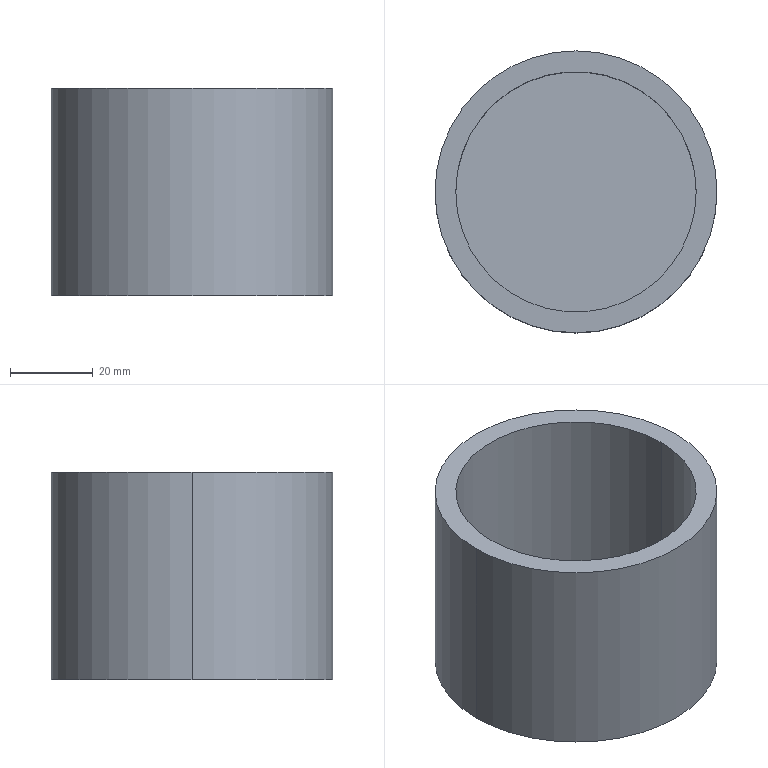Part | SolidWorks | features Extrusion 1, Shell 1 | 1 solid | 7 faces | box 68 x 68 x 50 mm | volume 62690 mm3 | cylinder 4 | plane 3 | commonest cylinder face diameters 58 x2 68 x2
STEP:
#1=CARTESIAN_POINT('',(-29.,0.,50.));
#2=VERTEX_POINT('',#1);
#3=CARTESIAN_POINT('',(29.,0.,50.));
#4=VERTEX_POINT('',#3);
#5=CARTESIAN_POINT('',(0.,0.,50.));
#6=DIRECTION('',(0.,0.,1.));
#7=DIRECTION('',(1.,0.,0.));
#8=AXIS2_PLACEMENT_3D('',#5,#6,#7);
#9=CIRCLE('',#8,29.);
#10=EDGE_CURVE('',#2,#4,#9,.T.);
#11=ORIENTED_EDGE('',*,*,#10,.T.);
#12=CARTESIAN_POINT('',(29.,0.,5.));
#13=VERTEX_POINT('',#12);
#14=CARTESIAN_POINT('',(29.,0.,50.));
#15=DIRECTION('',(0.,0.,-1.));
#16=VECTOR('',#15,1000.);
#17=LINE('',#14,#16);
#18=EDGE_CURVE('',#4,#13,#17,.T.);
#19=ORIENTED_EDGE('',*,*,#18,.T.);
#20=CARTESIAN_POINT('',(-29.,0.,5.));
#21=VERTEX_POINT('',#20);
#22=CARTESIAN_POINT('',(0.,0.,5.));
#23=DIRECTION('',(0.,0.,1.));
#24=DIRECTION('',(1.,0.,0.));
#25=AXIS2_PLACEMENT_3D('',#22,#23,#24);
#26=CIRCLE('',#25,29.);
#27=EDGE_CURVE('',#21,#13,#26,.T.);
#28=ORIENTED_EDGE('',*,*,#27,.F.);
#29=CARTESIAN_POINT('',(-29.,0.,50.));
#30=DIRECTION('',(0.,0.,-1.));
#31=VECTOR('',#30,1000.);
#32=LINE('',#29,#31);
#33=EDGE_CURVE('',#2,#21,#32,.T.);
#34=ORIENTED_EDGE('',*,*,#33,.F.);
#35=EDGE_LOOP('',(#11,#19,#28,#34));
#36=FACE_OUTER_BOUND('',#35,.T.);
#37=CARTESIAN_POINT('',(0.,0.,50.));
#38=DIRECTION('',(0.,0.,-1.));
#39=DIRECTION('',(-1.,0.,0.));
#40=AXIS2_PLACEMENT_3D('',#37,#38,#39);
#41=CYLINDRICAL_SURFACE('',#40,29.);
#42=ADVANCED_FACE('',(#36),#41,.F.);
#43=CARTESIAN_POINT('',(34.,0.,50.));
#44=VERTEX_POINT('',#43);
#45=CARTESIAN_POINT('',(-34.,0.,50.));
#46=VERTEX_POINT('',#45);
#47=CARTESIAN_POINT('',(0.,0.,50.));
#48=DIRECTION('',(0.,0.,1.));
#49=DIRECTION('',(1.,0.,0.));
#50=AXIS2_PLACEMENT_3D('',#47,#48,#49);
#51=CIRCLE('',#50,34.);
#52=EDGE_CURVE('',#44,#46,#51,.T.);
#53=ORIENTED_EDGE('',*,*,#52,.F.);
#54=CARTESIAN_POINT('',(34.,0.,0.));
#55=VERTEX_POINT('',#54);
#56=CARTESIAN_POINT('',(34.,0.,50.));
#57=DIRECTION('',(0.,0.,-1.));
#58=VECTOR('',#57,1000.);
#59=LINE('',#56,#58);
#60=EDGE_CURVE('',#44,#55,#59,.T.);
#61=ORIENTED_EDGE('',*,*,#60,.T.);
#62=CARTESIAN_POINT('',(-34.,0.,0.));
#63=VERTEX_POINT('',#62);
#64=CARTESIAN_POINT('',(0.,0.,0.));
#65=DIRECTION('',(0.,0.,1.));
#66=DIRECTION('',(1.,0.,0.));
#67=AXIS2_PLACEMENT_3D('',#64,#65,#66);
#68=CIRCLE('',#67,34.);
#69=EDGE_CURVE('',#55,#63,#68,.T.);
#70=ORIENTED_EDGE('',*,*,#69,.T.);
#71=CARTESIAN_POINT('',(-34.,0.,50.));
#72=DIRECTION('',(0.,0.,-1.));
#73=VECTOR('',#72,1000.);
#74=LINE('',#71,#73);
#75=EDGE_CURVE('',#46,#63,#74,.T.);
#76=ORIENTED_EDGE('',*,*,#75,.F.);
#77=EDGE_LOOP('',(#53,#61,#70,#76));
#78=FACE_OUTER_BOUND('',#77,.T.);
#79=CARTESIAN_POINT('',(0.,0.,50.));
#80=DIRECTION('',(0.,0.,-1.));
#81=DIRECTION('',(-1.,0.,0.));
#82=AXIS2_PLACEMENT_3D('',#79,#80,#81);
#83=CYLINDRICAL_SURFACE('',#82,34.);
#84=ADVANCED_FACE('',(#78),#83,.T.);
#85=ORIENTED_EDGE('',*,*,#60,.F.);
#86=CARTESIAN_POINT('',(0.,0.,50.));
#87=DIRECTION('',(0.,0.,1.));
#88=DIRECTION('',(1.,0.,0.));
#89=AXIS2_PLACEMENT_3D('',#86,#87,#88);
#90=CIRCLE('',#89,34.);
#91=EDGE_CURVE('',#46,#44,#90,.T.);
#92=ORIENTED_EDGE('',*,*,#91,.F.);
#93=ORIENTED_EDGE('',*,*,#75,.T.);
#94=CARTESIAN_POINT('',(0.,0.,0.));
#95=DIRECTION('',(0.,0.,1.));
#96=DIRECTION('',(1.,0.,0.));
#97=AXIS2_PLACEMENT_3D('',#94,#95,#96);
#98=CIRCLE('',#97,34.);
#99=EDGE_CURVE('',#63,#55,#98,.T.);
#100=ORIENTED_EDGE('',*,*,#99,.T.);
#101=EDGE_LOOP('',(#85,#92,#93,#100));
#102=FACE_OUTER_BOUND('',#101,.T.);
#103=CARTESIAN_POINT('',(0.,0.,50.));
#104=DIRECTION('',(0.,0.,-1.));
#105=DIRECTION('',(-1.,0.,0.));
#106=AXIS2_PLACEMENT_3D('',#103,#104,#105);
#107=CYLINDRICAL_SURFACE('',#106,34.);
#108=ADVANCED_FACE('',(#102),#107,.T.);
#109=ORIENTED_EDGE('',*,*,#10,.F.);
#110=CARTESIAN_POINT('',(0.,0.,50.));
#111=DIRECTION('',(0.,0.,1.));
#112=DIRECTION('',(1.,0.,0.));
#113=AXIS2_PLACEMENT_3D('',#110,#111,#112);
#114=CIRCLE('',#113,29.);
#115=EDGE_CURVE('',#4,#2,#114,.T.);
#116=ORIENTED_EDGE('',*,*,#115,.F.);
#117=EDGE_LOOP('',(#109,#116));
#118=FACE_BOUND('',#117,.T.);
#119=ORIENTED_EDGE('',*,*,#91,.T.);
#120=ORIENTED_EDGE('',*,*,#52,.T.);
#121=EDGE_LOOP('',(#119,#120));
#122=FACE_OUTER_BOUND('',#121,.T.);
#123=CARTESIAN_POINT('',(0.,0.,50.));
#124=DIRECTION('',(0.,0.,1.));
#125=DIRECTION('',(1.,0.,0.));
#126=AXIS2_PLACEMENT_3D('',#123,#124,#125);
#127=PLANE('',#126);
#128=ADVANCED_FACE('',(#118,#122),#127,.T.);
#129=ORIENTED_EDGE('',*,*,#99,.F.);
#130=ORIENTED_EDGE('',*,*,#69,.F.);
#131=EDGE_LOOP('',(#129,#130));
#132=FACE_OUTER_BOUND('',#131,.T.);
#133=CARTESIAN_POINT('',(0.,0.,0.));
#134=DIRECTION('',(0.,0.,1.));
#135=DIRECTION('',(1.,0.,0.));
#136=AXIS2_PLACEMENT_3D('',#133,#134,#135);
#137=PLANE('',#136);
#138=ADVANCED_FACE('',(#132),#137,.F.);
#139=ORIENTED_EDGE('',*,*,#18,.F.);
#140=ORIENTED_EDGE('',*,*,#115,.T.);
#141=ORIENTED_EDGE('',*,*,#33,.T.);
#142=CARTESIAN_POINT('',(0.,0.,5.));
#143=DIRECTION('',(0.,0.,1.));
#144=DIRECTION('',(1.,0.,0.));
#145=AXIS2_PLACEMENT_3D('',#142,#143,#144);
#146=CIRCLE('',#145,29.);
#147=EDGE_CURVE('',#13,#21,#146,.T.);
#148=ORIENTED_EDGE('',*,*,#147,.F.);
#149=EDGE_LOOP('',(#139,#140,#141,#148));
#150=FACE_OUTER_BOUND('',#149,.T.);
#151=CARTESIAN_POINT('',(0.,0.,50.));
#152=DIRECTION('',(0.,0.,-1.));
#153=DIRECTION('',(-1.,0.,0.));
#154=AXIS2_PLACEMENT_3D('',#151,#152,#153);
#155=CYLINDRICAL_SURFACE('',#154,29.);
#156=ADVANCED_FACE('',(#150),#155,.F.);
#157=ORIENTED_EDGE('',*,*,#27,.T.);
#158=ORIENTED_EDGE('',*,*,#147,.T.);
#159=EDGE_LOOP('',(#157,#158));
#160=FACE_OUTER_BOUND('',#159,.T.);
#161=CARTESIAN_POINT('',(0.,0.,5.));
#162=DIRECTION('',(0.,0.,1.));
#163=DIRECTION('',(1.,0.,0.));
#164=AXIS2_PLACEMENT_3D('',#161,#162,#163);
#165=PLANE('',#164);
#166=ADVANCED_FACE('',(#160),#165,.T.);
#167=CLOSED_SHELL('',(#42,#84,#108,#128,#138,#156,#166));
#168=MANIFOLD_SOLID_BREP('',#167);
#169=CARTESIAN_POINT('',(0.,0.,0.));
#170=DIRECTION('',(0.,0.,1.));
#171=DIRECTION('',(1.,0.,0.));
#172=AXIS2_PLACEMENT_3D('',#169,#170,#171);
#173=(LENGTH_UNIT()NAMED_UNIT(*)SI_UNIT(.MILLI.,.METRE.));
#174=UNCERTAINTY_MEASURE_WITH_UNIT(LENGTH_MEASURE(0.00001),#173,'','');
#175=(NAMED_UNIT(*)PLANE_ANGLE_UNIT()SI_UNIT($,.RADIAN.));
#176=(NAMED_UNIT(*)SI_UNIT($,.STERADIAN.)SOLID_ANGLE_UNIT());
#177=(GEOMETRIC_REPRESENTATION_CONTEXT(3)GLOBAL_UNCERTAINTY_ASSIGNED_CONTEXT((#174))GLOBAL_UNIT_ASSIGNED_CONTEXT((#173,#175,#176))REPRESENTATION_CONTEXT('',''));
#178=ADVANCED_BREP_SHAPE_REPRESENTATION('',(#168,#172),#177);